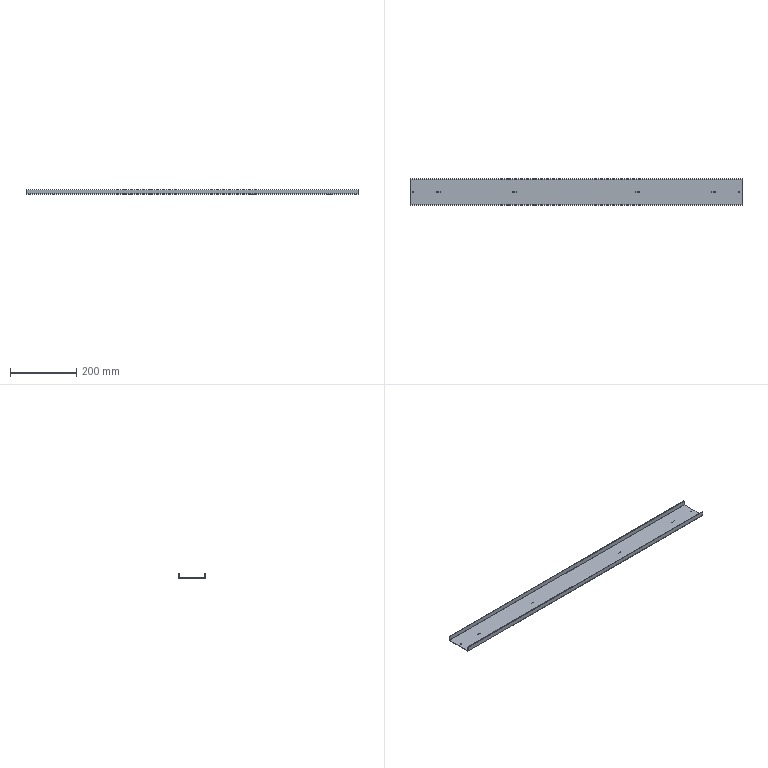Part | STEP file | FHD-021-001-P rack welded part P | 1 solid | 32 faces | box 1000 x 80 x 15 mm | volume 159142 mm3 | plane 26 | cylinder 6 | commonest cylinder face diameters 0.4 x2 2.5 x2 3.4 x2